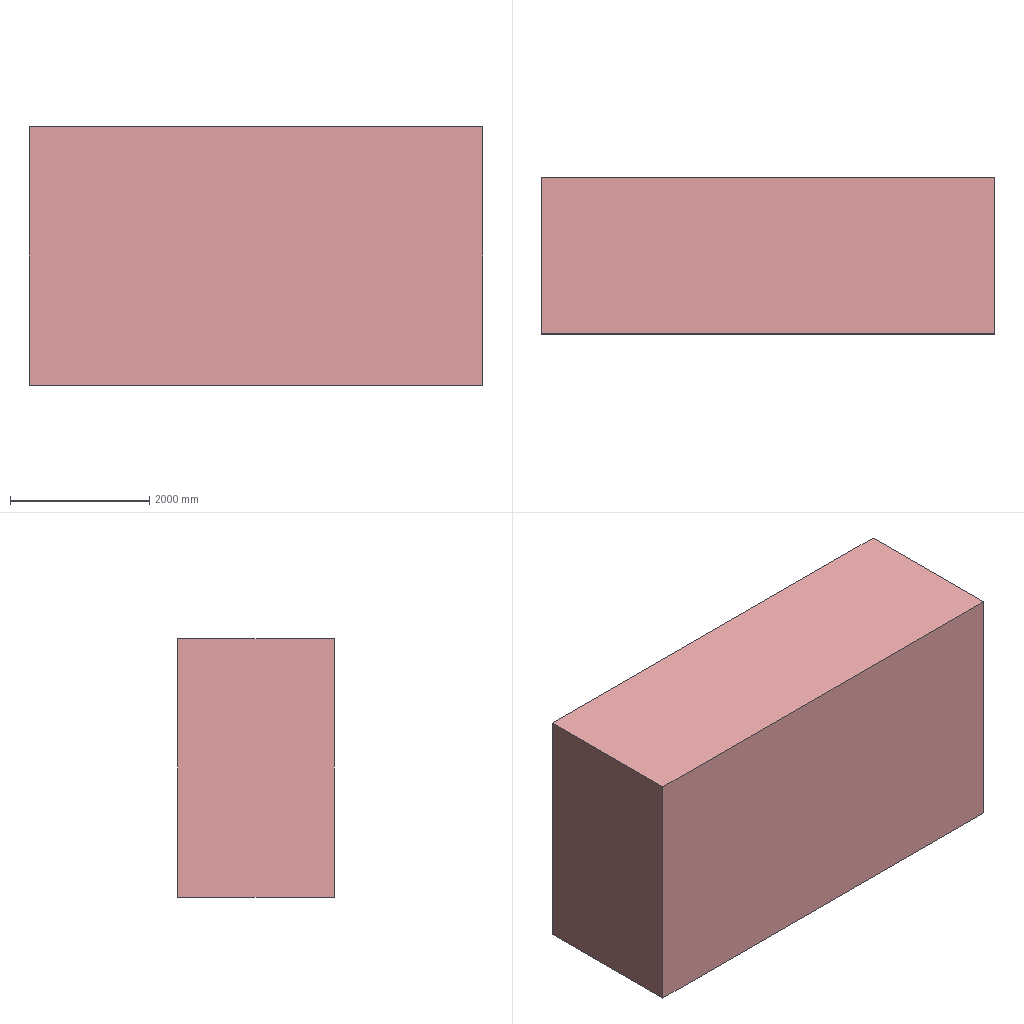Assembly | SolidWorks | 9 different items | 501 placed | box 6500 x 2240 x 3710 mm
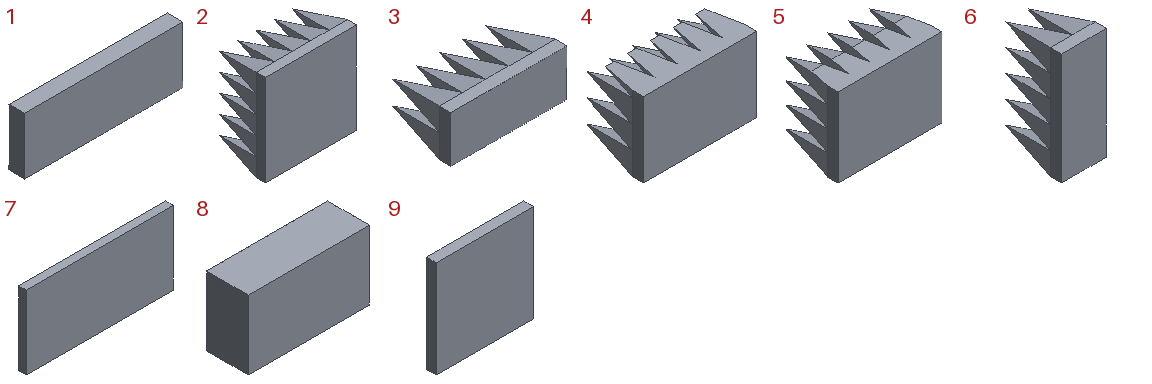Parts list (item | quantity | size | volume | features):
1 | x81 | 500 x 50 x 180 mm | 4500000 mm3 | features Extrusion 1
2 | x237 | 500 x 300 x 500 mm | 33333333 mm3 | features LPattern 2, Blend 1, Extrusion 1, ICE 1
3 | x1 | 500 x 300 x 200 mm | 13333333 mm3 | features LPattern 2, Blend 1, Extrusion 1, ICE 1
4 | x4 | 500 x 300 x 330 mm | 21650000 mm3 | features LPattern 2, Blend 1, Extrusion 1, ICE 1
5 | x38 | 500 x 300 x 380 mm | 25733333 mm3 | features LPattern 2, Blend 1, Extrusion 1, ICE 1
6 | x43 | 200 x 300 x 500 mm | 13333333 mm3 | features LPattern 2, Blend 1, Extrusion 1, ICE 1
7 | x8 | 1000 x 50 x 500 mm | 25000000 mm3 | features Extrusion 1
8 | x1 | 6500 x 2240 x 3710 mm | 2774520000 mm3 | features Extrusion 1, ICE 1
9 | x88 | 500 x 50 x 500 mm | 12500000 mm3 | features Extrusion 1
Mates (type | each side: item.copy, entity, surface, feature):
Coincident | 8.1 plane | assembly plane | 3 times
Coincident | 8.1 face plane Cut-Extrude 1 | 9.1 face plane Boss-Extrude 1 | 2 times
Coincident | 9.1 face plane Boss-Extrude 1 | 9.2 face plane Boss-Extrude 1 | 4 times
Coincident | 9.1 face plane Boss-Extrude 1 | 2.1 face plane Boss-Extrude 1 | 2 times
Coincident | 9.1 face plane Boss-Extrude 1 | 2.2 face plane Boss-Extrude 1 | 2 times
Coincident | 2.1 face plane Boss-Extrude 1 | 9.3 face plane Boss-Extrude 1
DistanceDim | 7.1 face plane Boss-Extrude 1 | 8.1 face plane Boss-Extrude 1
DistanceDim | 9.1 face plane Boss-Extrude 1 | 8.1 face plane Boss-Extrude 1
Coincident | 2.3 face plane Boss-Extrude 1 | assembly face | 2 times
Coincident | 9.2 edge | 2.3 face plane Boss-Extrude 1
Coincident | 2.3 face plane Boss-Extrude 1 | 2.4 face plane Boss-Extrude 1 | 2 times
Coincident | assembly face | 2.4 face plane Boss-Extrude 1 | 2 times
Coincident | 7.2 face plane Boss-Extrude 1 | 7.3 face plane Boss-Extrude 1 | 2 times
Coincident | 7.3 face plane Boss-Extrude 1 | 7.4 face plane Boss-Extrude 1 | 3 times
Coincident | 2.2 face plane Boss-Extrude 1 | 7.5 face plane Boss-Extrude 1
Coincident | 2.2 face plane Boss-Extrude 1 | 2.5 face plane Boss-Extrude 1
Coincident | 7.5 face plane Boss-Extrude 1 | 2.5 face plane Boss-Extrude 1
Coincident | 9.4 face plane Boss-Extrude 1 | 2.5 face plane Boss-Extrude 1
Coincident | 7.6 face plane Boss-Extrude 1 | 2.6 face plane Boss-Extrude 1
Coincident | 7.3 face plane Boss-Extrude 1 | 2.6 face plane Boss-Extrude 1
Coincident | 7.3 face plane Boss-Extrude 1 | 2.7 face plane Boss-Extrude 1
Coincident | 7.1 face plane Boss-Extrude 1 | 9.5 face plane Boss-Extrude 1
Coincident | 9.6 face plane Boss-Extrude 1 | assembly face
Coincident | 9.3 face plane Boss-Extrude 1 | 2.3 face plane Boss-Extrude 1 | 2 times
Coincident | 9.7 face plane Boss-Extrude 1 | 2.4 face plane Boss-Extrude 1
Coincident | 2.4 face plane Boss-Extrude 1 | 9.8 face plane Boss-Extrude 1 | 2 times
Coincident | 2.2 face plane Boss-Extrude 1 | 2.8 face plane Boss-Extrude 1
Coincident | 9.6 face plane Boss-Extrude 1 | 2.8 face plane Boss-Extrude 1
Coincident | 9.8 face plane Boss-Extrude 1 | 2.8 face plane Boss-Extrude 1
Coincident | 2.9 face plane Boss-Extrude 1 | 2.10 face plane Boss-Extrude 1 | 2 times
Coincident | 2.11 face plane Boss-Extrude 1 | 2.10 face plane Boss-Extrude 1
Coincident | 9.6 face plane Boss-Extrude 1 | 1.1 face plane Boss-Extrude 1 | 3 times
Coincident | 9.8 face plane Boss-Extrude 1 | 1.2 face plane Boss-Extrude 1 | 3 times
Coincident | 2.8 face plane Boss-Extrude 1 | 1.1 face plane Boss-Extrude 1 | 2 times
Coincident | 1.1 face plane Boss-Extrude 1 | 1.2 face plane Boss-Extrude 1
Coincident | 9.9 face plane Boss-Extrude 1 | 1.3 face plane Boss-Extrude 1 | 2 times
Coincident | 9.10 face plane Boss-Extrude 1 | 1.3 face plane Boss-Extrude 1
Coincident | 1.4 face plane Boss-Extrude 1 | 1.5 face plane Boss-Extrude 1 | 2 times
Coincident | 9.11 face plane Boss-Extrude 1 | 1.5 face plane Boss-Extrude 1
Coincident | 9.10 face plane Boss-Extrude 1 | 1.6 face plane Boss-Extrude 1 | 2 times
Coincident | 1.3 face plane Boss-Extrude 1 | 1.6 face plane Boss-Extrude 1
Coincident | 1.4 face plane Boss-Extrude 1 | 1.7 face plane Boss-Extrude 1 | 2 times
Coincident | 1.5 face plane Boss-Extrude 1 | 1.7 face plane Boss-Extrude 1
Coincident | 1.5 face plane Boss-Extrude 1 | 1.8 face plane Boss-Extrude 1
Coincident | 2.12 face plane Boss-Extrude 1 | 1.8 face plane Boss-Extrude 1
Coincident | 1.7 face plane Boss-Extrude 1 | 1.8 face plane Boss-Extrude 1
Coincident | 7.5 face plane Boss-Extrude 1 | 6.1 face plane Boss-Extrude 1
Coincident | 7.5 face plane Boss-Extrude 1 | 6.1 face plane Cut-Extrude 1
Coincident | 2.5 face plane Boss-Extrude 1 | 6.1 face plane Boss-Extrude 1
Coincident | 2.13 face plane Boss-Extrude 1 | 2.14 face plane Boss-Extrude 1
Coincident | 9.12 edge | 2.14 edge
Coincident | 9.13 face plane Boss-Extrude 1 | 2.14 face plane Boss-Extrude 1
Coincident | 2.14 face plane Boss-Extrude 1 | 9.14 face plane Boss-Extrude 1 | 2 times
Coincident | 1.9 face plane Boss-Extrude 1 | 9.14 face plane Boss-Extrude 1
Coincident | 2.14 face plane Boss-Extrude 1 | 2.15 face plane Boss-Extrude 1 | 3 times
Coincident | 2.15 face plane Boss-Extrude 1 | 9.15 face plane Boss-Extrude 1 | 3 times
Coincident | 1.10 face plane Boss-Extrude 1 | 1.9 face plane Boss-Extrude 1
Coincident | 9.14 face plane Boss-Extrude 1 | 1.9 face plane Boss-Extrude 1
Coincident | 1.11 face plane Boss-Extrude 1 | 1.12 face plane Boss-Extrude 1
Coincident | 9.15 face plane Boss-Extrude 1 | 1.12 face plane Boss-Extrude 1
Coincident | 1.13 face plane Boss-Extrude 1 | 1.12 face plane Boss-Extrude 1
Coincident | 1.12 face plane Boss-Extrude 1 | 1.14 face plane Boss-Extrude 1 | 2 times
Coincident | 1.13 face plane Boss-Extrude 1 | 1.14 face plane Boss-Extrude 1
Coincident | 9.16 face plane Boss-Extrude 1 | 1.15 face plane Boss-Extrude 1 | 2 times
Coincident | 9.14 face plane Boss-Extrude 1 | 1.15 face plane Boss-Extrude 1
Coincident | 1.14 face plane Boss-Extrude 1 | 1.16 face plane Boss-Extrude 1
Coincident | 9.17 face plane Boss-Extrude 1 | 1.16 face plane Boss-Extrude 1
Coincident | 1.12 face plane Boss-Extrude 1 | 1.16 face plane Boss-Extrude 1
Coincident | 2.16 face plane Boss-Extrude 1 | 2.17 face plane Boss-Extrude 1
Coincident | 9.17 face plane Boss-Extrude 1 | 2.17 face plane Boss-Extrude 1
Coincident | 2.18 edge | 2.17 face plane Boss-Extrude 1
Coincident | 2.17 face plane Boss-Extrude 1 | 1.17 face plane Boss-Extrude 1 | 2 times
Coincident | 9.17 face plane Boss-Extrude 1 | 1.17 face plane Boss-Extrude 1
Coincident | 2.19 face plane Boss-Extrude 1 | 2.20 face plane Boss-Extrude 1
Coincident | 9.18 face plane Boss-Extrude 1 | 2.20 face plane Boss-Extrude 1 | 2 times
Coincident | 2.21 face plane Boss-Extrude 1 | 2.22 face plane Boss-Extrude 1
Coincident | 9.5 face plane Boss-Extrude 1 | 2.22 face plane Boss-Extrude 1
Coincident | 7.1 face plane Boss-Extrude 1 | 2.22 face plane Boss-Extrude 1
Coincident | 9.19 face plane Boss-Extrude 1 | 6.2 face plane Boss-Extrude 1
Coincident | 9.4 face plane Boss-Extrude 1 | 6.2 face plane Boss-Extrude 1
Coincident | 2.1 face plane Boss-Extrude 1 | 6.2 face plane Boss-Extrude 1
Coincident | 2.23 face plane Boss-Extrude 1 | 5.1 face plane Cut-Extrude 2
Coincident | 2.23 face plane Boss-Extrude 1 | 5.1 face plane Boss-Extrude 1
Coincident | 9.6 face plane Boss-Extrude 1 | 5.1 face plane Boss-Extrude 1
Coincident | 2.24 face plane Boss-Extrude 1 | 4.1 face plane Boss-Extrude 1 | 2 times
Coincident | 9.20 face plane Boss-Extrude 1 | 4.1 face plane Boss-Extrude 1
Coincident | 4.1 face plane Boss-Extrude 1 | 4.2 face plane Boss-Extrude 1
Coincident | 2.25 face plane Boss-Extrude 1 | 4.2 face plane Boss-Extrude 1
Coincident | 9.9 face plane Boss-Extrude 1 | 4.2 face plane Boss-Extrude 1
Coincident | 2.1 face plane Boss-Extrude 1 | 6.3 face plane Boss-Extrude 1 | 2 times
Coincident | 2.1 face plane Boss-Extrude 1 | 6.3 face plane Cut-Extrude 1
Coincident | 6.3 face plane Boss-Extrude 1 | 6.4 face plane Boss-Extrude 1 | 2 times
Coincident | 9.6 face plane Boss-Extrude 1 | 6.4 face plane Boss-Extrude 1
Coincident | 2.26 face plane Boss-Extrude 1 | 5.2 face plane Cut-Extrude 2
Coincident | 2.26 face plane Boss-Extrude 1 | 5.2 face plane Boss-Extrude 1
Coincident | 9.2 face plane Boss-Extrude 1 | 6.5 face plane Boss-Extrude 1
Coincident | 2.27 face plane Boss-Extrude 1 | 6.5 face plane Boss-Extrude 1
DistanceDim | 5.2 face plane Boss-Extrude 1 | 9.6 face plane Boss-Extrude 1
Coincident | 5.2 face plane Boss-Extrude 1 | 6.5 face plane Boss-Extrude 1
Coincident | 5.3 face plane Boss-Extrude 1 | 5.4 face plane Boss-Extrude 1 | 2 times
DistanceDim | 5.4 face plane Boss-Extrude 1 | 1.18 face plane Boss-Extrude 1
Coincident | 6.6 face plane Boss-Extrude 1 | 6.7 face plane Boss-Extrude 1
Coincident | 5.4 face plane Boss-Extrude 1 | 6.7 face plane Boss-Extrude 1
Coincident | 2.28 edge | 6.7 face plane Boss-Extrude 1